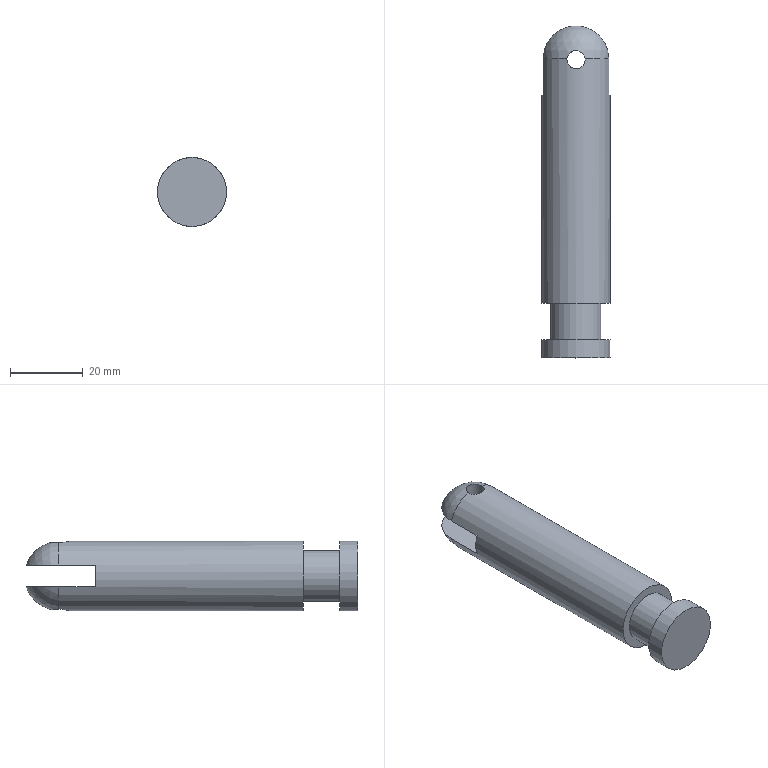Part | STEP file | 1-46.11 | 1 solid | 13 faces | box 19 x 91.264 x 19 mm | volume 21626 mm3 | plane 6 | cylinder 5 | sphere 2 | commonest cylinder face diameters 5 x2 19 x2 14 x1